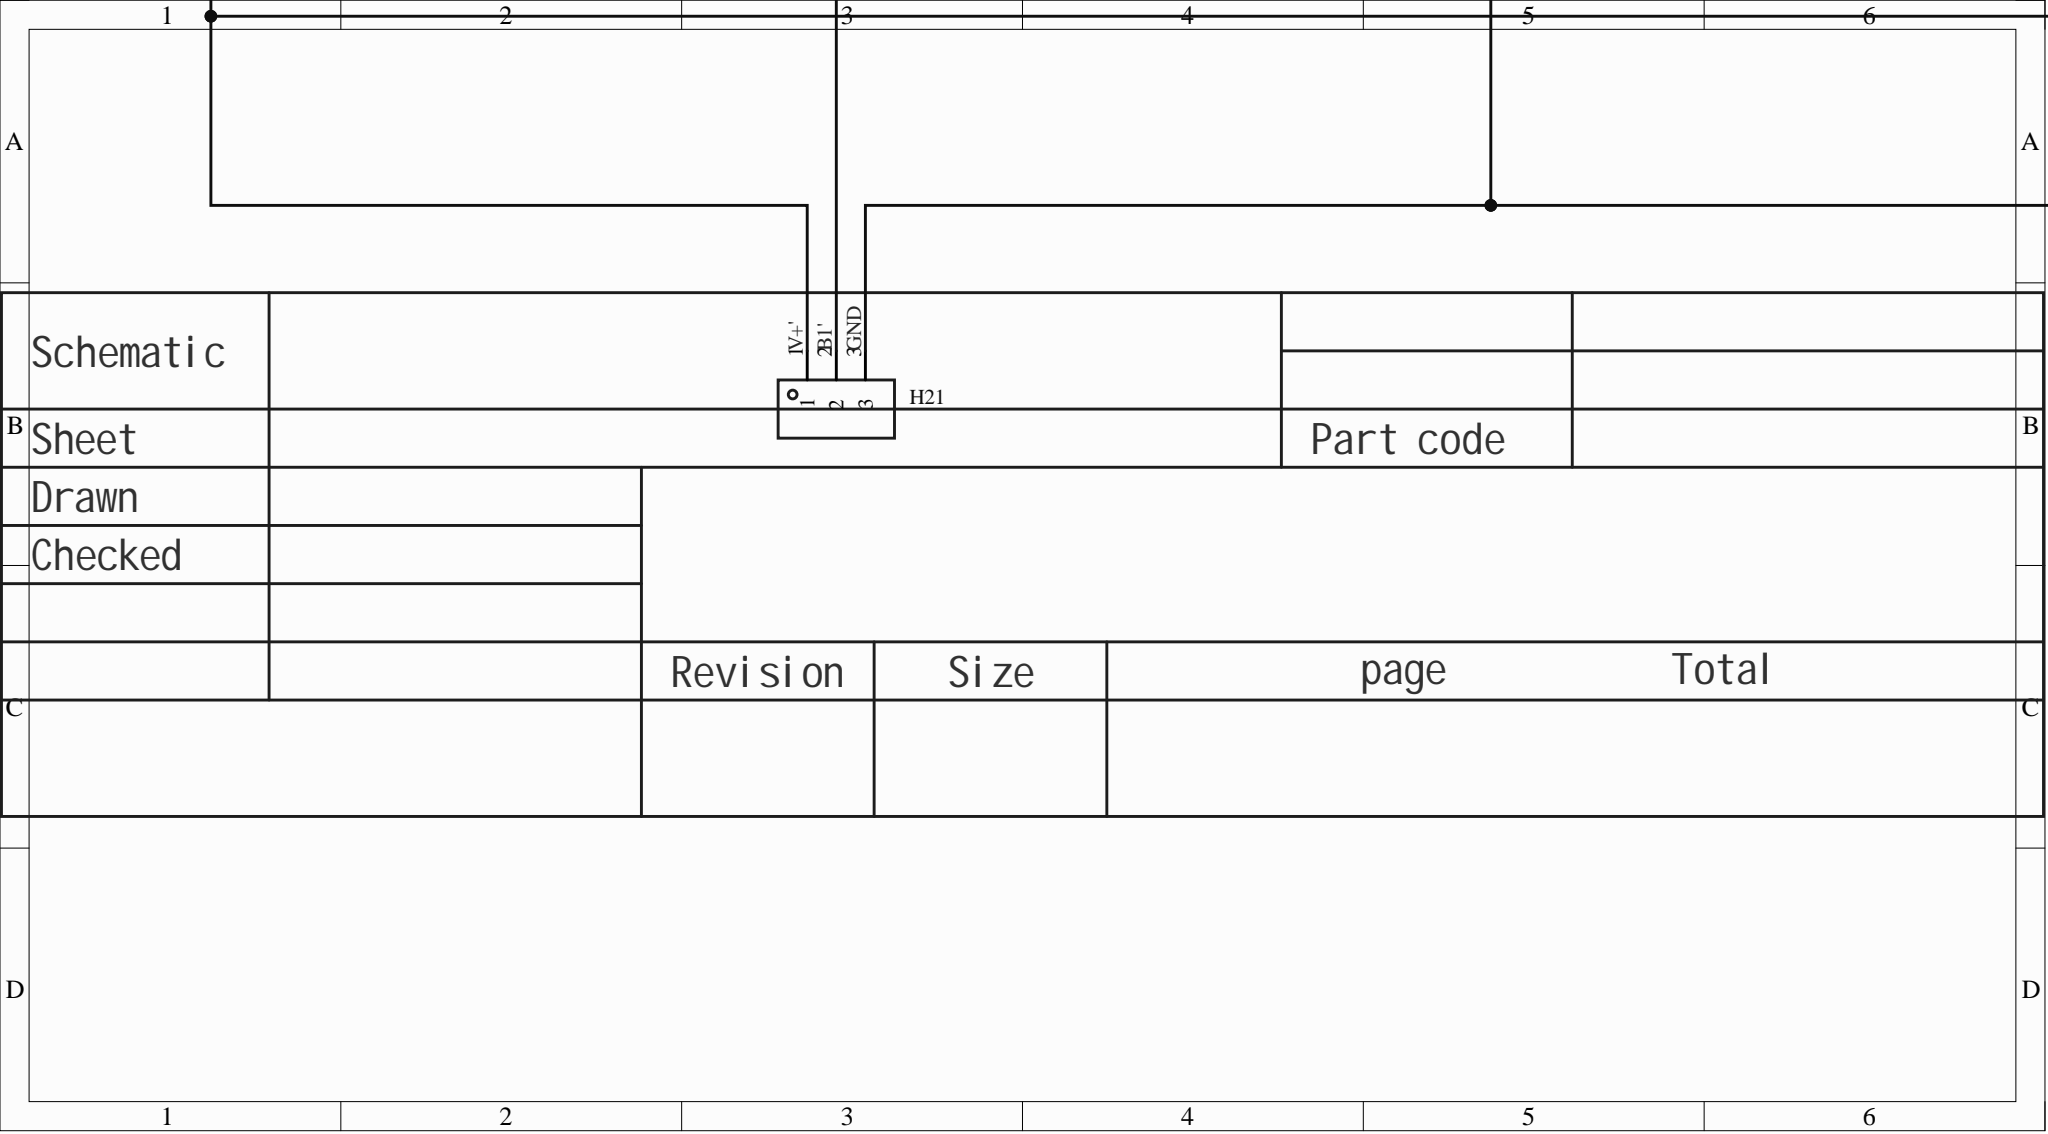Circuit board | Altium Designer | 303 parts | 159 nets
Bill of materials:
Comment,Description,Designator,Footprint,LibRef,Quantity
"0.1uF","","C1, C2, C4, C5, C6, C7, C8, C10, C11, C12, C13, C14, C15, C16, C18, C19, C20, C21, C22, C23, C24, C25, C26, C27, C28, C29, C30, C31, C32, C33, C34, C35, C36, C37, C38, C39, C41, C42, C43, C44, C45, C46, C47, C49, C50, C51, C52, C53, C54, C55, C56, C57, C58, C59, C60, C61, C62, C63","C0402","CAP_0402","58"
"0.02uF","","C9, C17, C40, C48","C0402","CAP_0402","4"
"","","H1, H21","HDR-TH_3P-P2.54-V-M","HDR-M_2.54_1x3P","2"
"","","H2, H3, H4, H5, H6, H7, H9, H10, H12, H13, H14, H15, H16, H17, H18, H19, H20, H22","HDR-TH_1P-V-M_XKB_X4611WV-01I-C28D40","HDR-M_2.54_1x1P","18"
"MMBT3906","transistor type: -; collector current (Ic): -; collector-emitter breakdown voltage (Vceo): -; power (Pd): -;","Q1, Q3, Q6, Q8, Q10, Q12, Q14, Q16, Q18, Q20, Q22, Q24, Q26, Q28, Q30, Q32, Q34, Q36, Q38, Q40, Q42, Q44, Q46, Q48, Q50, Q52, Q54, Q56, Q58, Q60, Q62, Q64","SOT-23-3_L2.9-W1.3-P1.90-LS2.4-BR","MMBT3906-13-01-F","32"
"MMBT3904","transistor type: NPN; collector current (Ic): 200mA; collector-emitter breakdown voltage (Vceo): 40V; power (Pd): 200mW; DC current gain (hFE@Ic,Vce): 100@10mA,1V;","Q2, Q4, Q5, Q7, Q9, Q11, Q13, Q15, Q17, Q19, Q21, Q23, Q25, Q27, Q29, Q31, Q33, Q35, Q37, Q39, Q41, Q43, Q45, Q47, Q49, Q51, Q53, Q55, Q57, Q59, Q61, Q63","SOT-23-3_L2.9-W1.3-P1.90-LS2.4-BR","MMBT3904(RANGE:100-300)","32"
"1","","R1, R5, R6, R10, R11, R12, R15, R18, R19, R22, R23, R26, R27, R30, R31, R33, R34, R37, R40, R41, R42, R45, R48, R49, R52, R53, R56, R57, R60, R61","R0402","Res_0402","30"
"2.2K","","R3, R4, R7, R9, R13, R14, R16, R17, R20, R24, R25, R28, R29, R32, R35, R36, R38, R39, R43, R44, R46, R47, R50, R54, R55, R58, R59, R62, R63","R0402","Res_0402","29"
"2.55K","","R21, R51","R0402","Res_0402","2"
"1K","","Rb1, Rb2, Rb3, Rb4, Rb5, Rb6, Rb7, Rb8, Rb9, Rb10, Rb11, Rb12, Rb13, Rb14, Rb15, Rb16, Rb17, Rb18, Rb19, Rb20, Rb21, Rb22, Rb23, Rb24, Rb25, Rb26, Rb27, Rb28, Rb29, Rb30, Rb31, Rb32","R0402","Res_0402","32"
"200K","","Rp1, Rp2, Rp3, Rp4, Rp5, Rp6, Rp7, Rp8, Rp9, Rp10, Rp11, Rp12, Rp13, Rp14, Rp15, Rp16, Rp17, Rp18, Rp19, Rp20, Rp21, Rp22, Rp23, Rp24, Rp25, Rp26, Rp27, Rp28, Rp29, Rp30, Rp31, Rp32","R0402","Res_0402","32"
"200","","Rs1, Rs2, Rs3, Rs4, Rs5, Rs6, Rs7, Rs8, Rs9, Rs10, Rs11, Rs12, Rs13, Rs14, Rs15, Rs16, Rs17, Rs18, Rs19, Rs20, Rs21, Rs22, Rs23, Rs24, Rs25, Rs26, Rs27, Rs28, Rs29, Rs30, Rs31, Rs32","R0402","Res_0402","32"
Netlist (Protel format):
[
C1
C0402
0.1uF



]
[
C2
C0402
0.1uF



]
[
C4
C0402
0.1uF



]
[
C5
C0402
0.1uF



]
[
C6
C0402
0.1uF



]
[
C7
C0402
0.1uF



]
[
C8
C0402
0.1uF



]
[
C9
C0402
0.02uF



]
[
C10
C0402
0.1uF



]
[
C11
C0402
0.1uF



]
[
C12
C0402
0.1uF



]
[
C13
C0402
0.1uF



]
[
C14
C0402
0.1uF



]
[
C15
C0402
0.1uF



]
[
C16
C0402
0.1uF



]
[
C17
C0402
0.02uF



]
[
C18
C0402
0.1uF



]
[
C19
C0402
0.1uF



]
[
C20
C0402
0.1uF



]
[
C21
C0402
0.1uF



]
[
C22
C0402
0.1uF



]
[
C23
C0402
0.1uF



]
[
C24
C0402
0.1uF



]
[
C25
C0402
0.1uF



]
[
C26
C0402
0.1uF



]
[
C27
C0402
0.1uF



]
[
C28
C0402
0.1uF



]
[
C29
C0402
0.1uF



]
[
C30
C0402
0.1uF



]
[
C31
C0402
0.1uF



]
[
C32
C0402
0.1uF



]
[
C33
C0402
0.1uF



]
[
C34
C0402
0.1uF



]
[
C35
C0402
0.1uF



]
[
C36
C0402
0.1uF



]
[
C37
C0402
0.1uF



]
[
C38
C0402
0.1uF



]
[
C39
C0402
0.1uF



]
[
C40
C0402
0.02uF



]
[
C41
C0402
0.1uF



]
[
C42
C0402
0.1uF



]
[
C43
C0402
0.1uF



]
[
C44
C0402
0.1uF



]
[
C45
C0402
0.1uF



]
[
C46
C0402
0.1uF



]
[
C47
C0402
0.1uF



]
[
C48
C0402
0.02uF



]
[
C49
C0402
0.1uF



]
[
C50
C0402
0.1uF



]
[
C51
C0402
0.1uF



]
[
C52
C0402
0.1uF



]
[
C53
C0402
0.1uF



]
[
C54
C0402
0.1uF



]
[
C55
C0402
0.1uF



]
[
C56
C0402
0.1uF



]
[
C57
C0402
0.1uF



]
[
C58
C0402
0.1uF



]
[
C59
C0402
0.1uF



]
[
C60
C0402
0.1uF



]
[
C61
C0402
0.1uF



]
[
C62
C0402
0.1uF



]
[
C63
C0402
0.1uF



]
[
H1
HDR-TH_3P-P2.54-V-M




]
[
H2
HDR-TH_1P-V-M_XKB_X4611WV-01I-C28D40




]
[
H3
HDR-TH_1P-V-M_XKB_X4611WV-01I-C28D40




]
[
H4
HDR-TH_1P-V-M_XKB_X4611WV-01I-C28D40




]
[
H5
HDR-TH_1P-V-M_XKB_X4611WV-01I-C28D40




]
[
H6
HDR-TH_1P-V-M_XKB_X4611WV-01I-C28D40




]
[
H7
HDR-TH_1P-V-M_XKB_X4611WV-01I-C28D40




]
[
H9
HDR-TH_1P-V-M_XKB_X4611WV-01I-C28D40




]
[
H10
HDR-TH_1P-V-M_XKB_X4611WV-01I-C28D40




]
[
H12
HDR-TH_1P-V-M_XKB_X4611WV-01I-C28D40




]
[
H13
HDR-TH_1P-V-M_XKB_X4611WV-01I-C28D40




]
[
H14
HDR-TH_1P-V-M_XKB_X4611WV-01I-C28D40




]
[
H15
HDR-TH_1P-V-M_XKB_X4611WV-01I-C28D40




]
[
H16
HDR-TH_1P-V-M_XKB_X4611WV-01I-C28D40




]
[
H17
HDR-TH_1P-V-M_XKB_X4611WV-01I-C28D40




]
[
H18
HDR-TH_1P-V-M_XKB_X4611WV-01I-C28D40




]
[
H19
HDR-TH_1P-V-M_XKB_X4611WV-01I-C28D40




]
[
H20
HDR-TH_1P-V-M_XKB_X4611WV-01I-C28D40




]
[
H21
HDR-TH_3P-P2.54-V-M




]
[
H22
HDR-TH_1P-V-M_XKB_X4611WV-01I-C28D40




]
[
Q1
SOT-23-3_L2.9-W1.3-P1.90-LS2.4-BR
MMBT3906



]
[
Q2
SOT-23-3_L2.9-W1.3-P1.90-LS2.4-BR
MMBT3904



]
[
Q3
SOT-23-3_L2.9-W1.3-P1.90-LS2.4-BR
MMBT3906



]
[
Q4
SOT-23-3_L2.9-W1.3-P1.90-LS2.4-BR
MMBT3904



]
[
Q5
SOT-23-3_L2.9-W1.3-P1.90-LS2.4-BR
MMBT3904



]
[
Q6
SOT-23-3_L2.9-W1.3-P1.90-LS2.4-BR
MMBT3906



]
[
Q7
SOT-23-3_L2.9-W1.3-P1.90-LS2.4-BR
MMBT3904



]
[
Q8
SOT-23-3_L2.9-W1.3-P1.90-LS2.4-BR
MMBT3906



]
[
Q9
SOT-23-3_L2.9-W1.3-P1.90-LS2.4-BR
MMBT3904



]
[
Q10
SOT-23-3_L2.9-W1.3-P1.90-LS2.4-BR
MMBT3906



]
[
Q11
SOT-23-3_L2.9-W1.3-P1.90-LS2.4-BR
MMBT3904



]
[
Q12
SOT-23-3_L2.9-W1.3-P1.90-LS2.4-BR
MMBT3906



]
[
Q13
SOT-23-3_L2.9-W1.3-P1.90-LS2.4-BR
MMBT3904



]
[
Q14
SOT-23-3_L2.9-W1.3-P1.90-LS2.4-BR
MMBT3906



]
[
Q15
SOT-23-3_L2.9-W1.3-P1.90-LS2.4-BR
MMBT3904



]
[
Q16
SOT-23-3_L2.9-W1.3-P1.90-LS2.4-BR
MMBT3906



]
[
Q17
SOT-23-3_L2.9-W1.3-P1.90-LS2.4-BR
MMBT3904



]
[
Q18
SOT-23-3_L2.9-W1.3-P1.90-LS2.4-BR
MMBT3906



]
[
Q19
SOT-23-3_L2.9-W1.3-P1.90-LS2.4-BR
MMBT3904



]
[
Q20
SOT-23-3_L2.9-W1.3-P1.90-LS2.4-BR
MMBT3906



]
[
Q21
SOT-23-3_L2.9-W1.3-P1.90-LS2.4-BR
MMBT3904



]
[
Q22
SOT-23-3_L2.9-W1.3-P1.90-LS2.4-BR
MMBT3906



]
[
Q23
SOT-23-3_L2.9-W1.3-P1.90-LS2.4-BR
MMBT3904



]
[
Q24
SOT-23-3_L2.9-W1.3-P1.90-LS2.4-BR
MMBT3906



]
[
Q25
SOT-23-3_L2.9-W1.3-P1.90-LS2.4-BR
MMBT3904



]
[
Q26
SOT-23-3_L2.9-W1.3-P1.90-LS2.4-BR
MMBT3906



]
[
Q27
SOT-23-3_L2.9-W1.3-P1.90-LS2.4-BR
MMBT3904



]
[
Q28
SOT-23-3_L2.9-W1.3-P1.90-LS2.4-BR
MMBT3906



]
[
Q29
SOT-23-3_L2.9-W1.3-P1.90-LS2.4-BR
MMBT3904



]
[
Q30
SOT-23-3_L2.9-W1.3-P1.90-LS2.4-BR
MMBT3906



]
[
Q31
SOT-23-3_L2.9-W1.3-P1.90-LS2.4-BR
MMBT3904



]
[
Q32
SOT-23-3_L2.9-W1.3-P1.90-LS2.4-BR
MMBT3906



]
[
Q33
SOT-23-3_L2.9-W1.3-P1.90-LS2.4-BR
MMBT3904



]
[
Q34
SOT-23-3_L2.9-W1.3-P1.90-LS2.4-BR
MMBT3906



]
[
Q35
SOT-23-3_L2.9-W1.3-P1.90-LS2.4-BR
MMBT3904



]
[
Q36
SOT-23-3_L2.9-W1.3-P1.90-LS2.4-BR
MMBT3906



]
[
Q37
SOT-23-3_L2.9-W1.3-P1.90-LS2.4-BR
MMBT3904



]
[
Q38
SOT-23-3_L2.9-W1.3-P1.90-LS2.4-BR
MMBT3906



]
[
Q39
SOT-23-3_L2.9-W1.3-P1.90-LS2.4-BR
MMBT3904



]
[
Q40
SOT-23-3_L2.9-W1.3-P1.90-LS2.4-BR
MMBT3906



]
[
Q41
SOT-23-3_L2.9-W1.3-P1.90-LS2.4-BR
MMBT3904



]
[
Q42
SOT-23-3_L2.9-W1.3-P1.90-LS2.4-BR
MMBT3906



]
[
Q43
SOT-23-3_L2.9-W1.3-P1.90-LS2.4-BR
MMBT3904



]
[
Q44
SOT-23-3_L2.9-W1.3-P1.90-LS2.4-BR
MMBT3906



]
[
Q45
SOT-23-3_L2.9-W1.3-P1.90-LS2.4-BR
MMBT3904



]
[
Q46
SOT-23-3_L2.9-W1.3-P1.90-LS2.4-BR
MMBT3906



]
[
Q47
SOT-23-3_L2.9-W1.3-P1.90-LS2.4-BR
MMBT3904



]
[
Q48
SOT-23-3_L2.9-W1.3-P1.90-LS2.4-BR
MMBT3906



]
[
Q49
SOT-23-3_L2.9-W1.3-P1.90-LS2.4-BR
MMBT3904



]
[
Q50
SOT-23-3_L2.9-W1.3-P1.90-LS2.4-BR
MMBT3906



]
[
Q51
SOT-23-3_L2.9-W1.3-P1.90-LS2.4-BR
MMBT3904



]
[
Q52
SOT-23-3_L2.9-W1.3-P1.90-LS2.4-BR
MMBT3906



]
[
Q53
SOT-23-3_L2.9-W1.3-P1.90-LS2.4-BR
MMBT3904



]
[
Q54
SOT-23-3_L2.9-W1.3-P1.90-LS2.4-BR
MMBT3906



]
[
Q55
SOT-23-3_L2.9-W1.3-P1.90-LS2.4-BR
MMBT3904



]
[
Q56
SOT-23-3_L2.9-W1.3-P1.90-LS2.4-BR
MMBT3906



]
[
Q57
SOT-23-3_L2.9-W1.3-P1.90-LS2.4-BR
MMBT3904



]
[
Q58
SOT-23-3_L2.9-W1.3-P1.90-LS2.4-BR
MMBT3906



]
[
Q59
SOT-23-3_L2.9-W1.3-P1.90-LS2.4-BR
MMBT3904



]
[
Q60
SOT-23-3_L2.9-W1.3-P1.90-LS2.4-BR
MMBT3906



]
[
Q61
SOT-23-3_L2.9-W1.3-P1.90-LS2.4-BR
MMBT3904



]
[
Q62
SOT-23-3_L2.9-W1.3-P1.90-LS2.4-BR
MMBT3906



]
[
Q63
SOT-23-3_L2.9-W1.3-P1.90-LS2.4-BR
MMBT3904



]
[
Q64
SOT-23-3_L2.9-W1.3-P1.90-LS2.4-BR
MMBT3906



]
[
R1
R0402
1



]
[
R3
R0402
2.2K



]
[
R4
R0402
2.2K



]
[
R5
R0402
1



]
[
R6
R0402
1



]
[
R7
R0402
2.2K



]
[
R9
R0402
2.2K



]
[
R10
R0402
1



]
[
R11
R0402
1



]
[
R12
R0402
1



]
[
R13
R0402
2.2K



]
[
R14
R0402
2.2K



]
[
R15
R0402
1



]
[
R16
R0402
2.2K



]
[
R17
R0402
2.2K



]
[
R18
R0402
1



]
[
R19
R0402
1



]
[
R20
R0402
2.2K



]
[
R21
R0402
2.55K



]
[
R22
R0402
1



]
[
R23
R0402
1



]
[
R24
R0402
2.2K



]
[
R25
R0402
2.2K



]
[
R26
R0402
1



]
[
R27
R0402
1



]
[
R28
R0402
2.2K



]
[
R29
R0402
2.2K



]
[
R30
R0402
1



]
[
R31
R0402
1



]
[
R32
R0402
2.2K



]
[
R33
R0402
1



]
[
R34
R0402
1



]
[
R35
R0402
2.2K



]
[
R36
R0402
2.2K



]
[
R37
R0402
1



]
[
R38
R0402
2.2K



]
[
R39
R0402
2.2K



]
[
R40
R0402
1



]
[
R41
R0402
1



]
[
R42
R0402
1



]
[
R43
R0402
2.2K



]
[
R44
R0402
2.2K



]
[
R45
R0402
1



]
[
R46
R0402
2.2K



]
[
R47
R0402
2.2K



]
[
R48
R0402
1



]
[
R49
R0402
1



]
[
R50
R0402
2.2K



]
[
R51
R0402
2.55K



]
[
R52
R0402
1



]
[
R53
R0402
1



]
[
R54
R0402
2.2K



]
[
R55
R0402
2.2K



]
[
R56
R0402
1



]
[
R57
R0402
1



]
[
R58
R0402
2.2K



]
[
R59
R0402
2.2K



]
[
R60
R0402
1



]
[
R61
R0402
1



]
[
R62
R0402
2.2K



]
[
R63
R0402
2.2K



]
[
Rb1
R0402
1K



]
[
Rb2
R0402
1K



]
[
Rb3
R0402
1K



]
[
Rb4
R0402
1K



]
[
Rb5
R0402
1K



]
[
Rb6
R0402
1K



]
[
Rb7
R0402
1K



]
[
Rb8
R0402
1K



]
[
Rb9
R0402
1K



]
[
Rb10
R0402
1K



]
[
Rb11
R0402
1K



]
[
Rb12
R0402
1K



]
[
Rb13
R0402
1K



]
[
Rb14
R0402
1K



]
[
Rb15
R0402
1K



]
[
Rb16
R0402
1K



]
[
Rb17
R0402
1K



]
[
Rb18
R0402
1K



]
[
Rb19
R0402
1K



]
[
Rb20
R0402
1K



]
[
Rb21
R0402
1K



]
[
Rb22
R0402
1K



]
[
Rb23
R0402
1K



]
[
Rb24
R0402
1K



]
[
Rb25
R0402
1K



]
[
Rb26
R0402
1K



]
[
Rb27
R0402
1K



]
[
Rb28
R0402
1K



]
[
Rb29
R0402
1K



]
[
Rb30
R0402
1K



]
[
Rb31
R0402
1K



]
[
Rb32
R0402
1K



]
[
Rp1
R0402
200K



]
[
Rp2
R0402
200K



]
[
Rp3
R0402
200K



]
[
Rp4
R0402
200K



]
[
Rp5
R0402
200K



]
[
Rp6
R0402
200K



]
[
Rp7
R0402
200K



]
[
Rp8
R0402
200K



]
[
Rp9
R0402
200K



]
[
Rp10
R0402
200K



]
[
Rp11
R0402
200K



]
[
Rp12
R0402
200K



]
[
Rp13
R0402
200K



]
[
Rp14
R0402
200K



]
[
Rp15
R0402
200K



]
[
Rp16
R0402
200K



]
[
Rp17
R0402
200K



]
[
Rp18
R0402
200K



]
[
Rp19
R0402
200K



]
[
Rp20
R0402
200K



]
[
Rp21
R0402
200K



]
[
Rp22
R0402
200K



]
[
Rp23
R0402
200K



]
[
Rp24
R0402
200K



]
[
Rp25
R0402
200K



]
[
Rp26
R0402
200K



]
[
Rp27
R0402
200K



]
[
Rp28
R0402
200K



]
[
Rp29
R0402
200K



]
[
Rp30
R0402
200K



]
[
Rp31
R0402
200K



]
[
Rp32
R0402
200K



]
[
Rs1
R0402
200



]
[
Rs2
R0402
200



]
[
Rs3
R0402
200



]
[
Rs4
R0402
200



]
[
Rs5
R0402
200



]
[
Rs6
R0402
200



]
[
Rs7
R0402
200



]
[
Rs8
R0402
200



]
[
Rs9
R0402
200



]
[
Rs10
R0402
200



]
[
Rs11
R0402
200



]
[
Rs12
R0402
200



]
[
Rs13
R0402
200



]
[
Rs14
R0402
200



]
[
Rs15
R0402
200



]
[
Rs16
R0402
200



]
[
Rs17
R0402
200



]
[
Rs18
R0402
200



]
[
Rs19
R0402
200



]
[
Rs20
R0402
200



]
[
Rs21
R0402
200



]
[
Rs22
R0402
200



]
[
Rs23
R0402
200



]
[
Rs24
R0402
200



]
[
Rs25
R0402
200



]
[
Rs26
R0402
200



]
[
Rs27
R0402
200



]
[
Rs28
R0402
200



]
[
Rs29
R0402
200



]
[
Rs30
R0402
200



]
[
Rs31
R0402
200



]
[
Rs32
R0402
200



]
(
VR2'
H14-1
Q47-2
Rp24-2
Rs24-1
)
(
VR2
H4-1
Q15-2
Rp8-2
Rs8-1
)
(
VR1'
H15-1
Q43-2
Rp22-2
Rs22-1
)
(
VR1
H5-1
Q11-2
Rp6-2
Rs6-1
)
(
VL2'
H13-1
Q39-2
Rp20-2
Rs20-1
)
(
VL2
H3-1
Q7-2
Rp4-2
Rs4-1
)
(
VL1'
H12-1
Q35-2
Rp18-2
Rs18-1
)
(
VL1
H2-1
Q4-2
Rp2-2
Rs2-1
)
(
V+
C4-1
C6-1
C10-1
C14-1
C18-1
C22-1
C26-1
C30-1
C31-1
C32-1
C33-1
C37-1
C41-1
C45-1
C49-1
C53-1
C57-1
C61-1
H1-1
H21-1
Q3-2
Q6-2
Q10-2
Q14-2
Q18-2
Q22-2
Q26-2
Q30-2
Q32-2
Q34-2
Q38-2
Q42-2
Q46-2
Q50-2
Q54-2
Q58-2
Q62-2
R4-1
R9-1
R13-1
R17-1
R20-1
R25-1
R29-1
R35-1
R39-1
R43-1
R47-1
R50-1
R55-1
R59-1
R63-1
Rp1-1
Rp3-1
Rp5-1
Rp7-1
Rp9-1
Rp11-1
Rp13-1
Rp15-1
Rp16-1
Rp17-1
Rp19-1
Rp21-1
Rp23-1
Rp25-1
Rp27-1
Rp29-1
Rp31-1
)
(
V4'
H19-1
Q63-2
Rp32-2
Rs32-1
)
(
V4
H10-1
Q31-2
Rp16-2
Rs16-1
)
(
V3'
H18-1
Q59-2
Rp30-2
Rs30-1
)
(
V3
H9-1
Q27-2
Rp14-2
Rs14-1
)
(
V2'
H17-1
Q55-2
Rp28-2
Rs28-1
)
(
V2
H7-1
Q23-2
Rp12-2
Rs12-1
)
(
V1'
H16-1
Q51-2
Rp26-2
Rs26-1
)
(
V1
H6-1
Q19-2
Rp10-2
Rs10-1
)
(
NetQ63_3
Q63-3
Q64-1
Rb32-2
)
(
NetQ63_1
Q63-1
Q64-3
Rb32-1
)
(
NetQ61_3
Q61-3
Q62-1
Rb31-2
)
(
NetQ61_2
Q61-2
Rp31-2
Rs31-1
)
(
NetQ61_1
Q61-1
Q62-3
Rb31-1
)
(
NetQ59_3
Q59-3
Q60-1
Rb30-2
)
(
NetQ59_1
Q59-1
Q60-3
Rb30-1
)
(
NetQ57_3
Q57-3
Q58-1
Rb29-2
)
(
NetQ57_2
Q57-2
Rp29-2
Rs29-1
)
(
NetQ57_1
Q57-1
Q58-3
Rb29-1
)
(
NetQ55_3
Q55-3
Q56-1
Rb28-2
)
(
NetQ55_1
Q55-1
Q56-3
Rb28-1
)
(
NetQ53_3
Q53-3
Q54-1
Rb27-2
)
(
NetQ53_2
Q53-2
Rp27-2
Rs27-1
)
(
NetQ53_1
Q53-1
Q54-3
Rb27-1
)
(
NetQ51_3
Q51-3
Q52-1
Rb26-2
)
(
NetQ51_1
Q51-1
Q52-3
Rb26-1
)
(
NetQ49_3
Q49-3
Q50-1
Rb25-2
)
(
NetQ49_2
Q49-2
Rp25-2
Rs25-1
)
(
NetQ49_1
Q49-1
Q50-3
Rb25-1
)
(
NetQ47_3
Q47-3
Q48-1
Rb24-2
)
(
NetQ47_1
Q47-1
Q48-3
Rb24-1
)
(
NetQ45_3
Q45-3
Q46-1
Rb23-2
)
(
NetQ45_2
Q45-2
Rp23-2
Rs23-1
)
(
NetQ45_1
Q45-1
Q46-3
Rb23-1
)
(
NetQ43_3
Q43-3
Q44-1
Rb22-2
)
(
NetQ43_1
Q43-1
Q44-3
Rb22-1
)
(
NetQ41_3
Q41-3
Q42-1
Rb21-2
)
(
NetQ41_2
Q41-2
Rp21-2
Rs21-1
)
(
NetQ41_1
Q41-1
Q42-3
Rb21-1
)
(
NetQ39_3
Q39-3
Q40-1
Rb20-2
)
(
NetQ39_1
Q39-1
Q40-3
Rb20-1
)
(
NetQ37_3
Q37-3
Q38-1
Rb19-2
)
(
NetQ37_2
Q37-2
Rp19-2
Rs19-1
)
(
NetQ37_1
Q37-1
Q38-3
Rb19-1
)
(
NetQ35_3
Q35-3
Q36-1
Rb18-2
)
(
NetQ35_1
Q35-1
Q36-3
Rb18-1
)
(
NetQ33_3
Q33-3
Q34-1
Rb17-2
)
(
NetQ33_2
Q33-2
Rp17-2
Rs17-1
)
(
NetQ33_1
Q33-1
Q34-3
Rb17-1
)
(
NetQ31_3
Q31-3
Q32-1
Rb16-2
)
(
NetQ31_1
Q31-1
Q32-3
Rb16-1
)
(
NetQ29_3
Q29-3
Q30-1
Rb15-2
)
(
NetQ29_2
Q29-2
Rp15-2
Rs15-1
)
(
NetQ29_1
Q29-1
Q30-3
Rb15-1
)
(
NetQ27_3
Q27-3
Q28-1
Rb14-2
)
(
NetQ27_1
Q27-1
Q28-3
Rb14-1
)
(
NetQ25_3
Q25-3
Q26-1
Rb13-2
)
(
NetQ25_2
Q25-2
Rp13-2
Rs13-1
)
(
NetQ25_1
Q25-1
Q26-3
Rb13-1
)
(
NetQ23_3
Q23-3
Q24-1
Rb12-2
)
(
NetQ23_1
Q23-1
Q24-3
Rb12-1
)
(
NetQ21_3
Q21-3
Q22-1
Rb11-2
)
(
NetQ21_2
Q21-2
Rp11-2
Rs11-1
)
(
NetQ21_1
Q21-1
Q22-3
Rb11-1
)
(
NetQ19_3
Q19-3
Q20-1
Rb10-2
)
(
NetQ19_1
Q19-1
Q20-3
Rb10-1
)
(
NetQ17_3
Q17-3
Q18-1
Rb9-2
)
(
NetQ17_2
Q17-2
Rp9-2
Rs9-1
)
(
NetQ17_1
Q17-1
Q18-3
Rb9-1
)
(
NetQ15_3
Q15-3
Q16-1
Rb8-2
)
(
NetQ15_1
Q15-1
Q16-3
Rb8-1
)
(
NetQ13_3
Q13-3
Q14-1
Rb7-2
)
(
NetQ13_2
Q13-2
Rp7-2
Rs7-1
)
(
NetQ13_1
Q13-1
Q14-3
Rb7-1
)
(
NetQ11_3
Q11-3
Q12-1
Rb6-2
)
(
NetQ11_1
Q11-1
Q12-3
Rb6-1
)
(
NetQ9_3
Q9-3
Q10-1
Rb5-2
)
(
NetQ9_2
Q9-2
Rp5-2
Rs5-1
)
(
NetQ9_1
Q9-1
Q10-3
Rb5-1
)
(
NetQ7_3
Q7-3
Q8-1
Rb4-2
)
(
NetQ7_1
Q7-1
Q8-3
Rb4-1
)
(
NetQ5_3
Q5-3
Q6-1
Rb3-2
)
(
NetQ5_2
Q5-2
Rp3-2
Rs3-1
)
(
NetQ5_1
Q5-1
Q6-3
Rb3-1
)
(
NetQ2_3
Q2-3
Q3-1
Rb1-2
)
(
NetQ2_2
Q2-2
Rp1-2
Rs1-1
)
(
NetQ2_1
Q2-1
Q3-3
Rb1-1
)
(
NetQ1_3
Q1-3
Q4-1
Rb2-1
)
(
NetQ1_1
Q1-1
Q4-3
Rb2-2
)
(
NetC63_2
C63-2
R61-1
)
(
NetC62_1
C62-1
C63-1
Q64-2
R63-2
Rp32-1
)
(
NetC60_2
C60-2
R60-1
)
(
NetC60_1
C60-1
C61-2
R61-2
R62-1
Rs31-2
)
(
NetC59_2
C59-2
R57-1
)
(
NetC58_1
C58-1
C59-1
Q60-2
R59-2
R60-2
Rp30-1
)
(
NetC56_2
C56-2
R56-1
)
(
NetC56_1
C56-1
C57-2
R57-2
R58-1
Rs29-2
)
(
NetC55_2
C55-2
R53-1
)
(
NetC54_1
C54-1
C55-1
Q56-2
R55-2
R56-2
Rp28-1
)
(
NetC52_2
C52-2
R52-1
)
(
NetC52_1
C52-1
C53-2
R53-2
R54-1
Rs27-2
)
(
NetC51_2
C51-2
R49-1
)
(
NetC50_1
C50-1
C51-1
Q52-2
R50-2
R52-2
Rp26-1
)
(
NetC48_2
C48-2
R48-1
)
(
NetC47_2
C47-2
R45-1
)
(
NetC46_1
C46-1
C47-1
Q48-2
R47-2
R48-2
Rp24-1
)
(
NetC44_2
C44-2
R42-1
)
(
NetC44_1
C44-1
C45-2
R45-2
R46-1
Rs23-2
)
(
NetC43_2
C43-2
R41-1
)
(
NetC42_1
C42-1
C43-1
Q44-2
R42-2
R43-2
Rp22-1
)
(
NetC40_2
C40-2
R40-1
)
(
NetC40_1
C40-1
C48-1
C49-2
R49-2
R51-1
Rs25-2
)
(
NetC39_2
C39-2
R37-1
)
(
NetC38_1
C38-1
C39-1
Q40-2
R39-2
R40-2
Rp20-1
)
(
NetC36_2
C36-2
R34-1
)
(
NetC36_1
C36-1
C37-2
R37-2
R38-1
Rs19-2
)
(
NetC35_2
C35-2
R33-1
)
(
NetC34_1
C34-1
C35-1
Q36-2
R34-2
R35-2
Rp18-1
)
(
NetC32_2
C32-2
R31-1
)
(
NetC29_2
C29-2
R30-1
)
(
NetC29_1
C29-1
C30-2
R31-2
R32-1
Rs15-2
)
(
NetC28_2
C28-2
R27-1
)
(
NetC27_1
C27-1
C28-1
Q28-2
R29-2
R30-2
Rp14-1
)
(
NetC25_2
C25-2
R26-1
)
(
NetC25_1
C25-1
C26-2
R27-2
R28-1
Rs13-2
)
(
NetC24_2
C24-2
R23-1
)
(
NetC23_1
C23-1
C24-1
Q24-2
R25-2
R26-2
Rp12-1
)
(
NetC21_2
C21-2
R22-1
)
(
NetC21_1
C21-1
C22-2
R23-2
R24-1
Rs11-2
)
(
NetC20_2
C20-2
R19-1
)
(
NetC19_1
C19-1
C20-1
Q20-2
R20-2
R22-2
Rp10-1
)
(
NetC17_2
C17-2
R18-1
)
(
NetC16_2
C16-2
R15-1
)
(
NetC15_1
C15-1
C16-1
Q16-2
R17-2
R18-2
Rp8-1
)
(
NetC13_2
C13-2
R12-1
)
(
NetC13_1
C13-1
C14-2
R15-2
R16-1
Rs7-2
)
(
NetC12_2
C12-2
R11-1
)
(
NetC11_1
C11-1
C12-1
Q12-2
R12-2
R13-2
Rp6-1
)
(
NetC9_2
C9-2
R10-1
)
(
NetC9_1
C9-1
C17-1
C18-2
R19-2
R21-1
Rs9-2
)
(
NetC8_2
C8-2
R6-1
)
(
NetC7_1
C7-1
C8-1
Q8-2
R9-2
R10-2
Rp4-1
)
(
NetC2_2
C2-2
R1-1
)
(
NetC2_1
C2-1
C5-1
Q1-2
R4-2
R5-2
Rp2-1
)
(
NetC1_2
C1-2
R5-1
)
(
NetC1_1
C1-1
C6-2
R6-2
R7-1
Rs3-2
)
(
GND
C5-2
C7-2
C11-2
C15-2
C19-2
C23-2
C27-2
C31-2
C34-2
C38-2
C42-2
C46-2
C50-2
C54-2
C58-2
C62-2
H1-3
H21-3
R3-2
R7-2
R14-2
R16-2
R21-2
R24-2
R28-2
R32-2
R36-2
R38-2
R44-2
R46-2
R51-2
R54-2
R58-2
R62-2
Rs2-2
Rs4-2
Rs6-2
Rs8-2
Rs10-2
Rs12-2
Rs14-2
Rs16-2
Rs18-2
Rs20-2
Rs22-2
Rs24-2
Rs26-2
Rs28-2
Rs30-2
Rs32-2
)
(
B2'
C41-2
H22-1
R41-2
R44-1
Rs21-2
)
(
B2
C33-2
H20-1
R33-2
R36-1
Rs17-2
)
(
B1'
C10-2
H21-2
R11-2
R14-1
Rs5-2
)
(
B1
C4-2
H1-2
R1-2
R3-1
Rs1-2
)